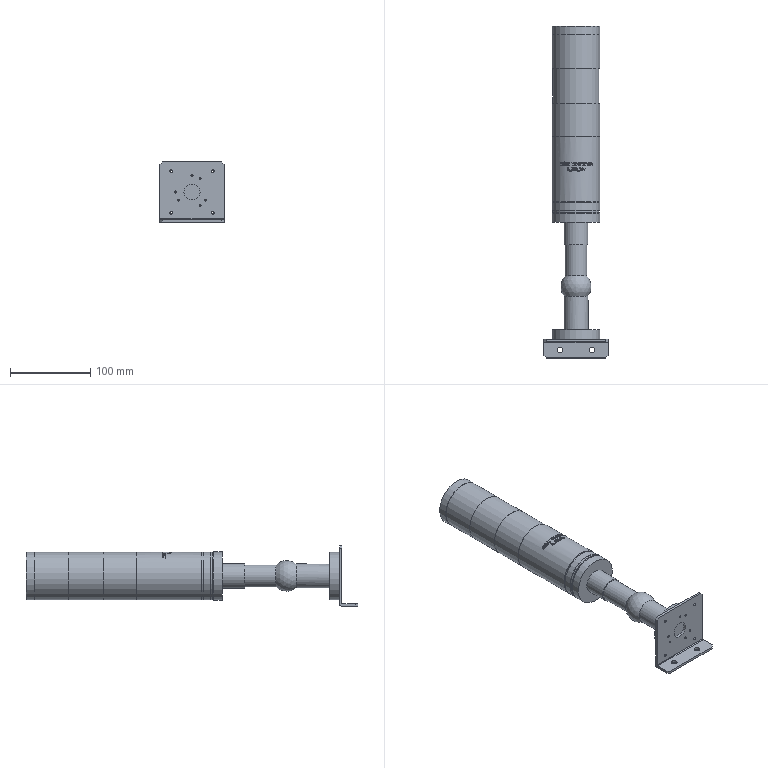Part | NX | 2 solids | 414 faces | box 80 x 414.5 x 75 mm | volume 829073 mm3 | plane 172 | spline 165 | cylinder 76 | sphere 1 | commonest cylinder face diameters 59.9 x31 59.7 x14 2.5 x6 3.3 x4 4.3 x3 11.3 x3